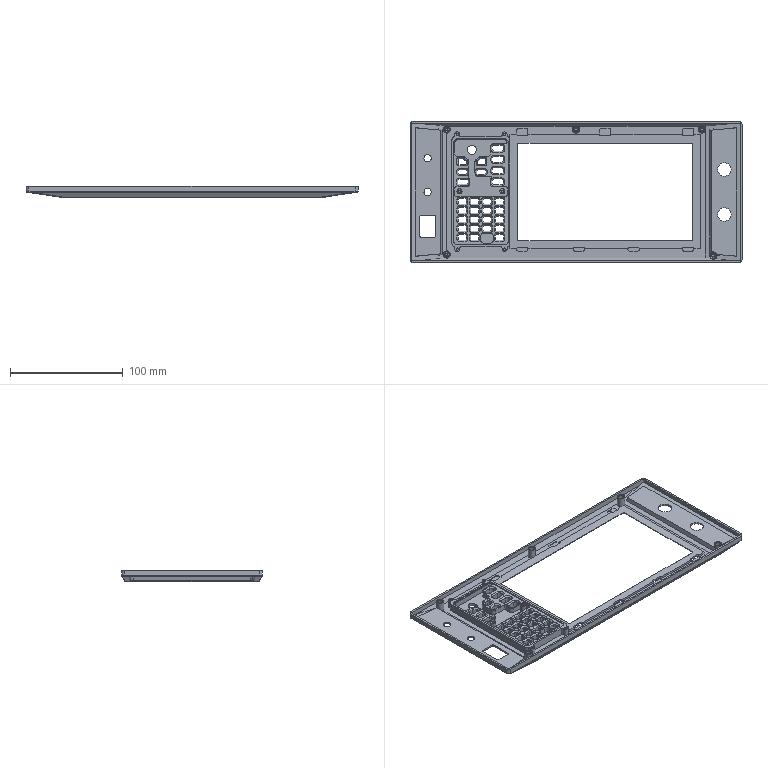NC program | NX | posted with a generic post | part box 295 x 125 x 10 mm
Lines 1 to 793 of 10380:
N10 G17 G21 G94 G90
(FLOOR_WALL_COPY , TOOL : D63)
N12 T01 M6
N14 G54
N16 G17 G0 G90 X-182. Y62.497 S6500 M3
N18 G43 Z30. H1
N20 Z4.
N22 G94 G1 Z1. F1250.
N24 X-179.
N26 X179.
N28 Y12.599
N30 X-179.
N32 Y-37.3
N34 X179.
N36 X182.
N38 Z4.
N40 G0 Z30.
N42 X-182. Y62.497
N44 Z3.
N46 G1 Z0.
N48 X-179.
N50 X179.
N52 Y12.599
N54 X-179.
N56 Y-37.3
N58 X179.
N60 X182.
N62 Z3.
N64 G0 Z30.
N66 M5
(ZLEVEL_PROFILE_1_COPY_1 , TOOL : D10)
N68 T10 M6
N70 G54
N72 G17 G0 G90 X52.07 Y-2.252 S9500 M3
N74 G43 Z30. H10
N76 Z1.5
N78 G94 G1 Y44.85 Z-0.969 F1000.
N80 X-103.94 F2200.
N82 Y-43.87
N84 X52.07
N86 Y44.85
N88 X-1.295 Z-1.9
N90 X-103.94
N92 Y-43.87
N94 X52.07
N96 Y44.85
N98 X52.05
N100 X-1.295
N102 Z-0.4
N104 G0 Z30.
N106 M5
(FLOOR_WALL_2 , TOOL : D6)
N108 T06 M6
N110 G54
N112 G17 G0 G90 X-148.5 Y-2.078 S9500 M3
N114 G43 Z30. H6
N116 Z1.132
N118 G94 G1 Z-0.368 F1000.
N120 X-145.8 Y-0.52
N122 G3 X-145.5 Y0. R0.6
N124 G1 Y59.168 F2500.
N126 X-144.95 Y59.118
N128 Y53.019
N130 X-124.211 Y51.104
N132 X-124.207 Y-51.099
N134 X-144.95 Y-53.019
N136 Y-59.118
N138 X-145.5 Y-59.168
N140 Y0.
N142 X-141.3
N144 Y48.464
N146 X-128.407 Y47.274
N148 Y-47.274
N150 X-141.3 Y-48.464
N152 Y0.
N154 X-137.1
N156 Y43.858
N158 X-132.607 Y43.444
N160 Y-43.444
N162 X-137.1 Y-43.858
N164 Y0.
N166 G3 X-137.4 Y0.52 R0.6
N168 G1 Z1.132
N170 G0 X-148.5 Y-2.078 Z0.594
N172 G1 Z-0.906 F1000.
N174 X-145.8 Y-0.52
N176 G3 X-145.5 Y0. R0.6
N178 G1 Y59.168 F2500.
N180 X-144.95 Y59.118
N182 Y53.019
N184 X-124.211 Y51.104
N186 X-124.207 Y-51.099
N188 X-144.95 Y-53.019
N190 Y-59.118
N192 X-145.5 Y-59.168
N194 Y0.
N196 X-141.3
N198 Y48.464
N200 X-128.407 Y47.274
N202 Y-47.274
N204 X-141.3 Y-48.464
N206 Y0.
N208 X-137.1
N210 Y43.858
N212 X-132.607 Y43.444
N214 Y-43.444
N216 X-137.1 Y-43.858
N218 Y0.
N220 G3 X-137.4 Y0.52 R0.6
N222 G1 Z0.594
N224 G0 X-148.5 Y-2.078 Z0.057
N226 G1 Z-1.443 F1000.
N228 X-145.8 Y-0.52
N230 G3 X-145.5 Y0. R0.6
N232 G1 Y59.168 F2500.
N234 X-144.95 Y59.118
N236 Y53.019
N238 X-124.211 Y51.104
N240 X-124.207 Y-51.099
N242 X-144.95 Y-53.019
N244 Y-59.118
N246 X-145.5 Y-59.168
N248 Y0.
N250 X-141.3
N252 Y48.464
N254 X-128.407 Y47.274
N256 Y-47.274
N258 X-141.3 Y-48.464
N260 Y0.
N262 X-137.1
N264 Y43.858
N266 X-132.607 Y43.444
N268 Y-43.444
N270 X-137.1 Y-43.858
N272 Y0.
N274 G3 X-137.4 Y0.52 R0.6
N276 G1 Z0.057
N278 G0 X-148.5 Y-2.078 Z-0.481
N280 G1 Z-1.981 F1000.
N282 X-145.8 Y-0.52
N284 G3 X-145.5 Y0. R0.6
N286 G1 Y59.168 F2500.
N288 X-144.95 Y59.118
N290 Y53.019
N292 X-124.211 Y51.104
N294 X-124.207 Y-51.099
N296 X-144.95 Y-53.019
N298 Y-59.118
N300 X-145.5 Y-59.168
N302 Y0.
N304 X-141.3
N306 Y48.464
N308 X-128.407 Y47.274
N310 Y-47.274
N312 X-141.3 Y-48.464
N314 Y0.
N316 X-137.1
N318 Y43.858
N320 X-132.607 Y43.444
N322 Y-43.444
N324 X-137.1 Y-43.858
N326 Y0.
N328 G3 X-137.4 Y0.52 R0.6
N330 G1 Z-0.481
N332 G0 X-148.5 Y-2.078 Z-1.018
N334 G1 Z-2.518 F1000.
N336 X-145.8 Y-0.52
N338 G3 X-145.5 Y0. R0.6
N340 G1 Y59.168 F2500.
N342 X-144.95 Y59.118
N344 Y53.019
N346 X-124.211 Y51.104
N348 X-124.207 Y-51.099
N350 X-144.95 Y-53.019
N352 Y-59.118
N354 X-145.5 Y-59.168
N356 Y0.
N358 X-141.3
N360 Y48.464
N362 X-128.407 Y47.274
N364 Y-47.274
N366 X-141.3 Y-48.464
N368 Y0.
N370 X-137.1
N372 Y43.858
N374 X-132.607 Y43.444
N376 Y-43.444
N378 X-137.1 Y-43.858
N380 Y0.
N382 G3 X-137.4 Y0.52 R0.6
N384 G1 Z-1.018
N386 G0 X-148.5 Y-2.078 Z-1.556
N388 G1 Z-3.056 F1000.
N390 X-145.8 Y-0.52
N392 G3 X-145.5 Y0. R0.6
N394 G1 Y59.168 F2500.
N396 X-144.95 Y59.118
N398 Y53.019
N400 X-124.211 Y51.104
N402 X-124.207 Y-51.099
N404 X-144.95 Y-53.019
N406 Y-59.118
N408 X-145.5 Y-59.168
N410 Y0.
N412 X-141.3
N414 Y48.464
N416 X-128.407 Y47.274
N418 Y-47.274
N420 X-141.3 Y-48.464
N422 Y0.
N424 X-137.1
N426 Y43.858
N428 X-132.607 Y43.444
N430 Y-43.444
N432 X-137.1 Y-43.858
N434 Y0.
N436 G3 X-137.4 Y0.52 R0.6
N438 G1 Z-1.556
N440 G0 X-148.5 Y-2.078 Z-2.093
N442 G1 Z-3.593 F1000.
N444 X-145.8 Y-0.52
N446 G3 X-145.5 Y0. R0.6
N448 G1 Y59.168 F2500.
N450 X-144.95 Y59.118
N452 Y53.019
N454 X-124.211 Y51.104
N456 X-124.207 Y-51.099
N458 X-144.95 Y-53.019
N460 Y-59.118
N462 X-145.5 Y-59.168
N464 Y0.
N466 X-141.3
N468 Y48.464
N470 X-128.407 Y47.274
N472 Y-47.274
N474 X-141.3 Y-48.464
N476 Y0.
N478 X-137.1
N480 Y43.858
N482 X-132.607 Y43.444
N484 Y-43.444
N486 X-137.1 Y-43.858
N488 Y0.
N490 G3 X-137.4 Y0.52 R0.6
N492 G1 Z-2.093
N494 G0 X-148.5 Y-2.078 Z-2.631
N496 G1 Z-4.131 F1000.
N498 X-145.8 Y-0.52
N500 G3 X-145.5 Y0. R0.6
N502 G1 Y54.274 F2500.
N504 G3 X-145.056 Y54.078 R0.6
N506 G1 X-144.95
N508 Y53.019
N510 X-124.211 Y51.104
N512 X-124.207 Y-51.099
N514 X-144.95 Y-53.019
N516 Y-54.076
N518 X-145.056
N520 G3 X-145.5 Y-54.273 R0.6
N522 G1 Y0.
N524 X-141.3
N526 Y48.464
N528 X-128.407 Y47.274
N530 Y-47.274
N532 X-141.3 Y-48.464
N534 Y0.
N536 X-137.1
N538 Y43.858
N540 X-132.607 Y43.444
N542 Y-43.444
N544 X-137.1 Y-43.858
N546 Y0.
N548 G3 X-137.4 Y0.52 R0.6
N550 G1 Z-2.631
N552 G0 Z30.
N554 X148.5 Y2.078
N556 Z1.132
N558 G1 Z-0.368 F1000.
N560 X145.8 Y0.52
N562 G3 X145.5 Y0. R0.6
N564 G1 Y-59.168 F2500.
N566 X144.95 Y-59.118
N568 Y-53.019
N570 X124.211 Y-51.104
N572 X124.207 Y51.099
N574 X144.95 Y53.019
N576 Y59.118
N578 X145.5 Y59.168
N580 Y0.
N582 X141.3
N584 Y-48.464
N586 X128.407 Y-47.274
N588 Y47.274
N590 X141.3 Y48.464
N592 Y0.
N594 X137.1
N596 Y-43.858
N598 X132.607 Y-43.444
N600 Y43.444
N602 X137.1 Y43.858
N604 Y0.
N606 G3 X137.4 Y-0.52 R0.6
N608 G1 Z1.132
N610 G0 X148.5 Y2.078 Z0.594
N612 G1 Z-0.906 F1000.
N614 X145.8 Y0.52
N616 G3 X145.5 Y0. R0.6
N618 G1 Y-59.168 F2500.
N620 X144.95 Y-59.118
N622 Y-53.019
N624 X124.211 Y-51.104
N626 X124.207 Y51.099
N628 X144.95 Y53.019
N630 Y59.118
N632 X145.5 Y59.168
N634 Y0.
N636 X141.3
N638 Y-48.464
N640 X128.407 Y-47.274
N642 Y47.274
N644 X141.3 Y48.464
N646 Y0.
N648 X137.1
N650 Y-43.858
N652 X132.607 Y-43.444
N654 Y43.444
N656 X137.1 Y43.858
N658 Y0.
N660 G3 X137.4 Y-0.52 R0.6
N662 G1 Z0.594
N664 G0 X148.5 Y2.078 Z0.057
N666 G1 Z-1.443 F1000.
N668 X145.8 Y0.52
N670 G3 X145.5 Y0. R0.6
N672 G1 Y-59.168 F2500.
N674 X144.95 Y-59.118
N676 Y-53.019
N678 X124.211 Y-51.104
N680 X124.207 Y51.099
N682 X144.95 Y53.019
N684 Y59.118
N686 X145.5 Y59.168
N688 Y0.
N690 X141.3
N692 Y-48.464
N694 X128.407 Y-47.274
N696 Y47.274
N698 X141.3 Y48.464
N700 Y0.
N702 X137.1
N704 Y-43.858
N706 X132.607 Y-43.444
N708 Y43.444
N710 X137.1 Y43.858
N712 Y0.
N714 G3 X137.4 Y-0.52 R0.6
N716 G1 Z0.057
N718 G0 X148.5 Y2.078 Z-0.481
N720 G1 Z-1.981 F1000.
N722 X145.8 Y0.52
N724 G3 X145.5 Y0. R0.6
N726 G1 Y-59.168 F2500.
N728 X144.95 Y-59.118
N730 Y-53.019
N732 X124.211 Y-51.104
N734 X124.207 Y51.099
N736 X144.95 Y53.019
N738 Y59.118
N740 X145.5 Y59.168
N742 Y0.
N744 X141.3
N746 Y-48.464
N748 X128.407 Y-47.274
N750 Y47.274
N752 X141.3 Y48.464
N754 Y0.
N756 X137.1
N758 Y-43.858
N760 X132.607 Y-43.444
N762 Y43.444
N764 X137.1 Y43.858
N766 Y0.
N768 G3 X137.4 Y-0.52 R0.6
N770 G1 Z-0.481
N772 G0 X148.5 Y2.078 Z-1.018
N774 G1 Z-2.518 F1000.
N776 X145.8 Y0.52
N778 G3 X145.5 Y0. R0.6
N780 G1 Y-59.168 F2500.
N782 X144.95 Y-59.118
N784 Y-53.019
N786 X124.211 Y-51.104
N788 X124.207 Y51.099
N790 X144.95 Y53.019
N792 Y59.118
N794 X145.5 Y59.168
N796 Y0.
N798 X141.3
N800 Y-48.464
N802 X128.407 Y-47.274
N804 Y47.274
N806 X141.3 Y48.464
N808 Y0.
N810 X137.1
N812 Y-43.858
N814 X132.607 Y-43.444
N816 Y43.444
N818 X137.1 Y43.858
N820 Y0.
N822 G3 X137.4 Y-0.52 R0.6
N824 G1 Z-1.018
N826 G0 X148.5 Y2.078 Z-1.556
N828 G1 Z-3.056 F1000.
N830 X145.8 Y0.52
N832 G3 X145.5 Y0. R0.6
N834 G1 Y-59.168 F2500.
N836 X144.95 Y-59.118
N838 Y-53.019
N840 X124.211 Y-51.104
N842 X124.207 Y51.099
N844 X144.95 Y53.019
N846 Y59.118
N848 X145.5 Y59.168
N850 Y0.
N852 X141.3
N854 Y-48.464
N856 X128.407 Y-47.274
N858 Y47.274
N860 X141.3 Y48.464
N862 Y0.
N864 X137.1
N866 Y-43.858
N868 X132.607 Y-43.444
N870 Y43.444
N872 X137.1 Y43.858
N874 Y0.
N876 G3 X137.4 Y-0.52 R0.6
N878 G1 Z-1.556
N880 G0 X148.5 Y2.078 Z-2.093
N882 G1 Z-3.593 F1000.
N884 X145.8 Y0.52
N886 G3 X145.5 Y0. R0.6
N888 G1 Y-59.168 F2500.
N890 X144.95 Y-59.118
N892 Y-53.019
N894 X124.211 Y-51.104
N896 X124.207 Y51.099
N898 X144.95 Y53.019
N900 Y59.118
N902 X145.5 Y59.168
N904 Y0.
N906 X141.3
N908 Y-48.464
N910 X128.407 Y-47.274
N912 Y47.274
N914 X141.3 Y48.464
N916 Y0.
N918 X137.1
N920 Y-43.858
N922 X132.607 Y-43.444
N924 Y43.444
N926 X137.1 Y43.858
N928 Y0.
N930 G3 X137.4 Y-0.52 R0.6
N932 G1 Z-2.093
N934 G0 X148.5 Y2.078 Z-2.631
N936 G1 Z-4.131 F1000.
N938 X145.8 Y0.52
N940 G3 X145.5 Y0. R0.6
N942 G1 Y-54.277 F2500.
N944 G3 X145.052 Y-54.076 R0.6
N946 G1 X144.95
N948 Y-53.019
N950 X124.211 Y-51.104
N952 X124.207 Y51.099
N954 X144.95 Y53.019
N956 Y54.078
N958 X145.052
N960 G3 X145.5 Y54.279 R0.6
N962 G1 Y0.
N964 X141.3
N966 Y-48.464
N968 X128.407 Y-47.274
N970 Y47.274
N972 X141.3 Y48.464
N974 Y0.
N976 X137.1
N978 Y-43.858
N980 X132.607 Y-43.444
N982 Y43.444
N984 X137.1 Y43.858
N986 Y0.
N988 G3 X137.4 Y-0.52 R0.6
N990 G1 Z-2.631
N992 G0 Z30.
(FLOOR_WALL_1_COPY , TOOL : D6)
N994 X147. Y52.314
N996 Z-2.731
N998 G1 Z-4.231 F1000.
N1000 X143.044
N1002 G3 X142.499 Y52.565 R0.6
N1004 G1 Y-52.565
N1006 X139.918 Y-52.326
N1008 Y52.326
N1010 X137.337 Y52.088
N1012 Y-52.088
N1014 X134.757 Y-51.85
N1016 Y51.85
N1018 X132.176 Y51.612
N1020 Y-51.612
N1022 X129.595 Y-51.374
N1024 Y51.374
N1026 X127.014 Y51.135
N1028 Y-51.135
N1030 X124.434 Y-50.897
N1032 Y50.897
N1034 Z-2.731
N1036 G0 Z30.
N1038 X147. Y51.542
N1040 Z-2.731
N1042 G1 Z-4.231
N1044 X146.045 Y52.892
N1046 G3 X145.5 Y53.143 R0.6
N1048 G1 X124.161 Y51.173
N1050 X124.135 Y51.169
N1052 X124.136 Y-51.169
N1054 X124.155 Y-51.173
N1056 X145.5 Y-53.143
N1058 G3 X146.045 Y-52.892 R0.6
N1060 G1 X147. Y-51.542
N1062 Z-2.731
N1064 G0 Z30.
N1066 X50.868 Y45.45
N1068 Z1.2
N1070 G1 Z-0.3
N1072 Y49.431
N1074 G3 X50.568 Y49.951 R0.6
N1076 G1 X-102.438
N1078 X-98.816 Y52.042
N1080 X46.946
N1082 X43.323 Y54.134
N1084 X-95.193
N1086 G3 X-95.493 Y53.614 R0.6
N1088 G1 Z1.2
N1090 G0 Z30.
N1092 X52.172 Y45.45
N1094 Z1.2
N1096 G1 Z-0.3
N1098 X53.87 Y46.43
N1100 G3 X54.17 Y46.95 R0.6
N1102 G1 Y48.218
N1104 X43.404 Y54.434
N1106 X-95.274
N1108 X-106.04 Y48.218
N1110 Y46.96
N1112 G3 X-105.74 Y46.44 R0.6
N1114 G1 X-104.025 Y45.45
N1116 Z1.2
N1118 G0 Z30.
N1120 X-147. Y-52.314
N1122 Z-2.731
N1124 G1 Z-4.231
N1126 X-143.044
N1128 G3 X-142.499 Y-52.565 R0.6
N1130 G1 Y52.565
N1132 X-139.918 Y52.326
N1134 Y-52.326
N1136 X-137.337 Y-52.088
N1138 Y52.088
N1140 X-134.757 Y51.85
N1142 Y-51.85
N1144 X-132.176 Y-51.612
N1146 Y51.612
N1148 X-129.595 Y51.374
N1150 Y-51.374
N1152 X-127.014 Y-51.135
N1154 Y51.135
N1156 X-124.434 Y50.897
N1158 Y-50.897
N1160 Z-2.731
N1162 G0 Z30.
N1164 X-147. Y-51.542
N1166 Z-2.731
N1168 G1 Z-4.231
N1170 X-146.045 Y-52.892
N1172 G3 X-145.5 Y-53.143 R0.6
N1174 G1 X-124.161 Y-51.173
N1176 X-124.135 Y-51.169
N1178 X-124.136 Y51.169
N1180 X-124.155 Y51.173
N1182 X-145.5 Y53.143
N1184 G3 X-146.045 Y52.892 R0.6
N1186 G1 X-147. Y51.542
N1188 Z-2.731
N1190 G0 Z30.
(ZLEVEL_PROFILE_1_COPY_COPY_COPY_COPY_COPY_COPY , TOOL : D6)
N1192 X50.914 Y-44.77
N1194 Z-0.3
N1196 G1 X51.434 Y-45.67
N1198 G3 X51.954 Y-45.97 R0.6
N1200 G1 X54.17 F2000.
N1202 Y-43.754
N1204 G3 X53.87 Y-43.234 R0.6
N1206 G1 X52.97 Y-42.714
N1208 G0 X50.914 Y-44.77 Z-0.725
N1210 G1 X51.434 Y-45.67 F1000.
N1212 G3 X51.954 Y-45.97 R0.6
N1214 G1 X54.17 F2000.
N1216 Y-43.754
N1218 G3 X53.87 Y-43.234 R0.6
N1220 G1 X52.97 Y-42.714
N1222 G0 X50.914 Y-44.77 Z-1.15
N1224 G1 X51.434 Y-45.67 F1000.
N1226 G3 X51.954 Y-45.97 R0.6
N1228 G1 X54.17 F2000.
N1230 Y-43.754
N1232 G3 X53.87 Y-43.234 R0.6
N1234 G1 X52.97 Y-42.714
N1236 G0 X50.914 Y-44.77 Z-1.575
N1238 G1 X51.434 Y-45.67 F1000.
N1240 G3 X51.954 Y-45.97 R0.6
N1242 G1 X54.17 F2000.
N1244 Y-43.754
N1246 G3 X53.87 Y-43.234 R0.6
N1248 G1 X52.97 Y-42.714
N1250 G0 X50.914 Y-44.77 Z-2.
N1252 G1 X51.434 Y-45.67 F1000.
N1254 G3 X51.954 Y-45.97 R0.6
N1256 G1 X54.17 F2000.
N1258 Y-43.754
N1260 G3 X53.87 Y-43.234 R0.6
N1262 G1 X52.97 Y-42.714
N1264 G0 Z30.
N1266 Y45.808
N1268 Z-0.3
N1270 G1 X53.87 Y46.327 F1000.
N1272 G3 X54.17 Y46.847 R0.6
N1274 G1 Y48.218 F2000.
N1276 X52.983 Y48.904
N1278 G3 X52.383 Y48.904 R0.6
N1280 G1 X51.483 Y48.384
N1282 G0 Z30.
N1284 X52.97 Y43.694
N1286 Z-0.725
N1288 G1 X53.87 Y44.214 F1000.
N1290 G3 X54.17 Y44.734 R0.6
N1292 G1 Y46.95 F2000.
N1294 X51.954
N1296 G3 X51.434 Y46.65 R0.6
N1298 G1 X50.914 Y45.75
N1300 G0 X52.97 Y43.694 Z-1.15
N1302 G1 X53.87 Y44.214 F1000.
N1304 G3 X54.17 Y44.734 R0.6
N1306 G1 Y46.95 F2000.
N1308 X51.954
N1310 G3 X51.434 Y46.65 R0.6
N1312 G1 X50.914 Y45.75
N1314 G0 X52.97 Y43.694 Z-1.575
N1316 G1 X53.87 Y44.214 F1000.
N1318 G3 X54.17 Y44.734 R0.6
N1320 G1 Y46.95 F2000.
N1322 X51.954
N1324 G3 X51.434 Y46.65 R0.6
N1326 G1 X50.914 Y45.75
N1328 G0 X52.97 Y43.694 Z-2.
N1330 G1 X53.87 Y44.214 F1000.
N1332 G3 X54.17 Y44.734 R0.6
N1334 G1 Y46.95 F2000.
N1336 X51.954
N1338 G3 X51.434 Y46.65 R0.6
N1340 G1 X50.914 Y45.75
N1342 G0 Z30.
N1344 X44.355 Y52.499
N1346 Z-0.3
N1348 G1 Y53.538 F1000.
N1350 G3 X44.055 Y54.058 R0.6
N1352 G1 X43.404 Y54.434 F2000.
N1354 X42.651
N1356 G3 X42.132 Y54.134 R0.6
N1358 G1 X41.612 Y53.234
N1360 G0 Z30.
N1362 X-93.482
N1364 Z-0.3
N1366 G1 X-94.002 Y54.134 F1000.
N1368 G3 X-94.521 Y54.434 R0.6
N1370 G1 X-95.274 F2000.
N1372 X-95.925 Y54.058
N1374 G3 X-96.225 Y53.538 R0.6
N1376 G1 Y52.499
N1378 G0 Z30.
N1380 X-103.353 Y48.384
N1382 Z-0.3
N1384 G1 X-104.253 Y48.904 F1000.
N1386 G3 X-104.853 Y48.904 R0.6
N1388 G1 X-106.04 Y48.218 F2000.
N1390 Y46.847
N1392 G3 X-105.74 Y46.327 R0.6
N1394 G1 X-104.84 Y45.808
N1396 G0 X-102.787 Y45.75 Z-0.725
N1398 G1 X-103.306 Y46.65 F1000.
N1400 G3 X-103.826 Y46.95 R0.6
N1402 G1 X-106.04 F2000.
N1404 Y44.734
N1406 G3 X-105.74 Y44.214 R0.6
N1408 G1 X-104.84 Y43.695
N1410 G0 X-102.784 Y45.75 Z-1.15
N1412 G1 X-103.304 Y46.65 F1000.
N1414 G3 X-103.824 Y46.95 R0.6
N1416 G1 X-106.04 F2000.
N1418 Y44.734
N1420 G3 X-105.74 Y44.214 R0.6
N1422 G1 X-104.84 Y43.694
N1424 G0 X-102.784 Y45.75 Z-1.575
N1426 G1 X-103.304 Y46.65 F1000.
N1428 G3 X-103.824 Y46.95 R0.6
N1430 G1 X-106.04 F2000.
N1432 Y44.734
N1434 G3 X-105.74 Y44.214 R0.6
N1436 G1 X-104.84 Y43.694
N1438 G0 X-102.784 Y45.75 Z-2.
N1440 G1 X-103.304 Y46.65 F1000.
N1442 G3 X-103.824 Y46.95 R0.6
N1444 G1 X-106.04 F2000.
N1446 Y44.734
N1448 G3 X-105.74 Y44.214 R0.6
N1450 G1 X-104.84 Y43.694
N1452 G0 Z30.
N1454 Y-42.714
N1456 Z-0.3
N1458 G1 X-105.74 Y-43.234 F1000.
N1460 G3 X-106.04 Y-43.754 R0.6
N1462 G1 Y-45.97 F2000.
N1464 X-103.824
N1466 G3 X-103.304 Y-45.67 R0.6
N1468 G1 X-102.784 Y-44.77
N1470 G0 X-104.84 Y-42.714 Z-0.725
N1472 G1 X-105.74 Y-43.234 F1000.
N1474 G3 X-106.04 Y-43.754 R0.6
N1476 G1 Y-45.97 F2000.
N1478 X-103.824
N1480 G3 X-103.304 Y-45.67 R0.6
N1482 G1 X-102.784 Y-44.77
N1484 G0 X-104.84 Y-42.714 Z-1.15
N1486 G1 X-105.74 Y-43.234 F1000.
N1488 G3 X-106.04 Y-43.754 R0.6
N1490 G1 Y-45.97 F2000.
N1492 X-103.824
N1494 G3 X-103.304 Y-45.67 R0.6
N1496 G1 X-102.784 Y-44.77
N1498 G0 X-104.84 Y-42.714 Z-1.575
N1500 G1 X-105.74 Y-43.234 F1000.
N1502 G3 X-106.04 Y-43.754 R0.6
N1504 G1 Y-45.97 F2000.
N1506 X-103.824
N1508 G3 X-103.304 Y-45.67 R0.6
N1510 G1 X-102.784 Y-44.77
N1512 G0 X-104.84 Y-42.714 Z-2.
N1514 G1 X-105.74 Y-43.234 F1000.
N1516 G3 X-106.04 Y-43.754 R0.6
N1518 G1 Y-45.97 F2000.
N1520 X-103.824
N1522 G3 X-103.304 Y-45.67 R0.6
N1524 G1 X-102.784 Y-44.77
N1526 G0 Z30.
(FLOOR_WALL_1_COPY_COPY , TOOL : D6)
N1528 X52.172 Y45.45
N1530 Z-0.5
N1532 G1 Z-2. F1000.
N1534 X53.87 Y46.43
N1536 G3 X54.17 Y46.95 R0.6
N1538 G1 X-106.04
N1540 Y-45.97
N1542 X54.17
N1544 Y46.95
N1546 G3 X53.65 Y46.65 R0.6
N1548 G1 X52.67 Y44.952
N1550 Z-0.5
N1552 G0 Z30.
N1554 M5